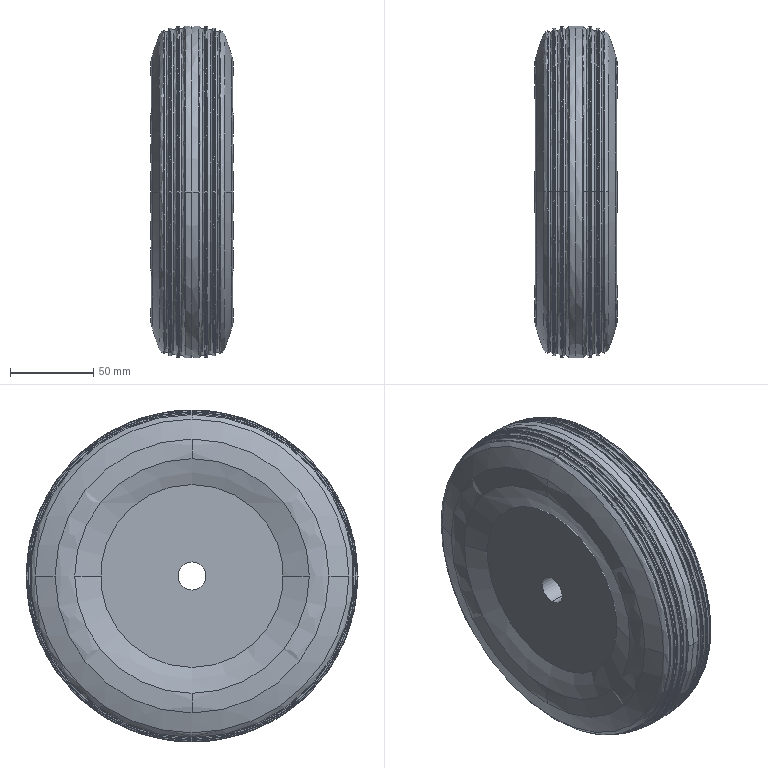Part | SolidWorks | features BaseBody 3 | 3 solids | 94 faces | box 50 x 200 x 200 mm | volume 2133858 mm3 | spline 70 | torus 10 | cylinder 10 | plane 4 | commonest cylinder face diameters 98.894 x4 110.246 x4 16.966 x2